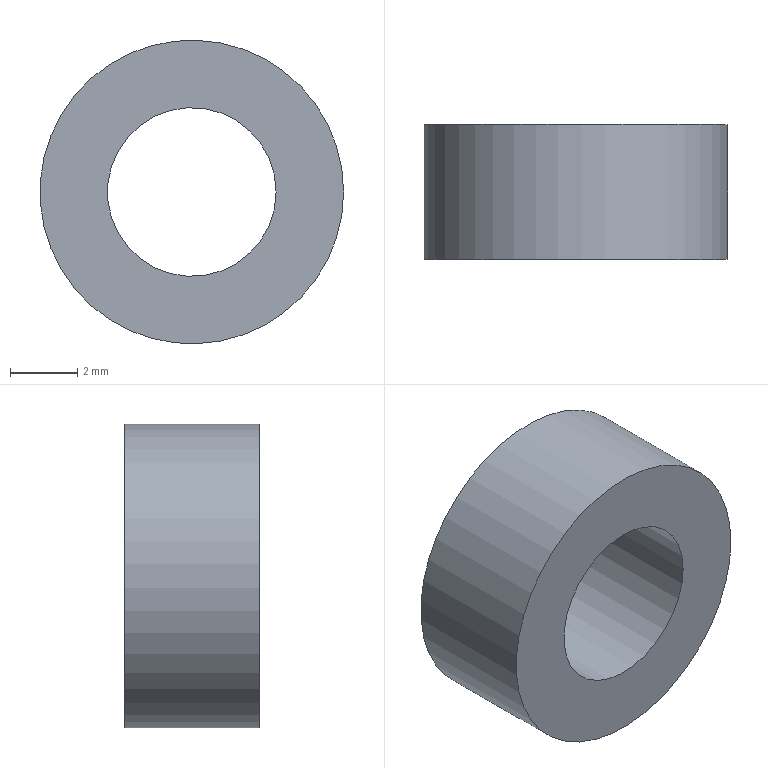Part | STEP file | 1-69.2 | 1 solid | 4 faces | box 9 x 4 x 9 mm | volume 175.929 mm3 | plane 2 | cylinder 2 | commonest cylinder face diameters 5 x1 9 x1
STEP:
#1=CARTESIAN_POINT('',(0.,0.,0.));
#2=DIRECTION('',(0.,0.,1.));
#3=DIRECTION('',(1.,0.,0.));
#4=AXIS2_PLACEMENT_3D('',#1,#2,#3);
#5=CARTESIAN_POINT('',(4.5,-2.,0.));
#6=VERTEX_POINT('',#5);
#7=CARTESIAN_POINT('',(0.,-2.,0.));
#8=DIRECTION('',(0.,-1.,0.));
#9=DIRECTION('',(1.,0.,0.));
#10=AXIS2_PLACEMENT_3D('',#7,#8,#9);
#11=CIRCLE('',#10,4.5);
#12=CARTESIAN_POINT('',(-1.206,-2.,0.));
#13=DIRECTION('',(0.,-1.,0.));
#14=DIRECTION('',(1.,0.,0.));
#15=AXIS2_PLACEMENT_3D('',#12,#13,#14);
#16=PLANE('',#15);
#17=CARTESIAN_POINT('',(1.206,0.));
#18=DIRECTION('',(1.,0.));
#19=AXIS2_PLACEMENT_2D('',#17,#18);
#20=CIRCLE('',#19,4.5);
#21=(GEOMETRIC_REPRESENTATION_CONTEXT(2)PARAMETRIC_REPRESENTATION_CONTEXT()REPRESENTATION_CONTEXT('',''));
#22=DEFINITIONAL_REPRESENTATION('',(#20),#21);
#23=PCURVE('',#16,#22);
#24=CARTESIAN_POINT('',(0.,-2.,0.));
#25=DIRECTION('',(0.,1.,0.));
#26=DIRECTION('',(1.,0.,0.));
#27=AXIS2_PLACEMENT_3D('',#24,#25,#26);
#28=CYLINDRICAL_SURFACE('',#27,4.5);
#29=CARTESIAN_POINT('',(6.283,0.));
#30=DIRECTION('',(-1.,0.));
#31=VECTOR('',#30,1.);
#32=LINE('',#29,#31);
#33=(GEOMETRIC_REPRESENTATION_CONTEXT(2)PARAMETRIC_REPRESENTATION_CONTEXT()REPRESENTATION_CONTEXT('',''));
#34=DEFINITIONAL_REPRESENTATION('',(#32),#33);
#35=PCURVE('',#28,#34);
#36=SURFACE_CURVE('',#11,(#23,#35),.PCURVE_S1.);
#37=EDGE_CURVE('',#6,#6,#36,.T.);
#38=ORIENTED_EDGE('',*,*,#37,.T.);
#39=EDGE_LOOP('',(#38));
#40=FACE_BOUND('',#39,.T.);
#41=CARTESIAN_POINT('',(2.5,-2.,0.));
#42=VERTEX_POINT('',#41);
#43=CARTESIAN_POINT('',(0.,-2.,0.));
#44=DIRECTION('',(0.,1.,0.));
#45=DIRECTION('',(1.,0.,0.));
#46=AXIS2_PLACEMENT_3D('',#43,#44,#45);
#47=CIRCLE('',#46,2.5);
#48=CARTESIAN_POINT('',(3.706,0.));
#49=CARTESIAN_POINT('',(3.706,-4.33));
#50=CARTESIAN_POINT('',(-0.04423,-2.165));
#51=CARTESIAN_POINT('',(-3.794,0.));
#52=CARTESIAN_POINT('',(-0.04423,2.165));
#53=CARTESIAN_POINT('',(3.706,4.33));
#54=CARTESIAN_POINT('',(3.706,0.));
#55=(BOUNDED_CURVE()B_SPLINE_CURVE(2,(#48,#49,#50,#51,#52,#53,#54),.UNSPECIFIED.,.T.,.F.)B_SPLINE_CURVE_WITH_KNOTS((1,2,2,2,2,1),(-2.094,0.,2.094,4.189,6.283,8.378),.UNSPECIFIED.)CURVE()GEOMETRIC_REPRESENTATION_ITEM()RATIONAL_B_SPLINE_CURVE((1.,0.5,1.,0.5,1.,0.5,1.))REPRESENTATION_ITEM(''));
#56=(GEOMETRIC_REPRESENTATION_CONTEXT(2)PARAMETRIC_REPRESENTATION_CONTEXT()REPRESENTATION_CONTEXT('',''));
#57=DEFINITIONAL_REPRESENTATION('',(#55),#56);
#58=PCURVE('',#16,#57);
#59=CARTESIAN_POINT('',(0.,-2.,0.));
#60=DIRECTION('',(0.,1.,0.));
#61=DIRECTION('',(1.,0.,0.));
#62=AXIS2_PLACEMENT_3D('',#59,#60,#61);
#63=CYLINDRICAL_SURFACE('',#62,2.5);
#64=CARTESIAN_POINT('',(0.,0.));
#65=DIRECTION('',(1.,0.));
#66=VECTOR('',#65,1.);
#67=LINE('',#64,#66);
#68=(GEOMETRIC_REPRESENTATION_CONTEXT(2)PARAMETRIC_REPRESENTATION_CONTEXT()REPRESENTATION_CONTEXT('',''));
#69=DEFINITIONAL_REPRESENTATION('',(#67),#68);
#70=PCURVE('',#63,#69);
#71=SURFACE_CURVE('',#47,(#58,#70),.PCURVE_S1.);
#72=EDGE_CURVE('',#42,#42,#71,.T.);
#73=ORIENTED_EDGE('',*,*,#72,.T.);
#74=EDGE_LOOP('',(#73));
#75=FACE_BOUND('',#74,.T.);
#76=ADVANCED_FACE('',(#40,#75),#16,.T.);
#77=CARTESIAN_POINT('',(4.5,2.,0.));
#78=VERTEX_POINT('',#77);
#79=CARTESIAN_POINT('',(0.,2.,0.));
#80=DIRECTION('',(0.,-1.,0.));
#81=DIRECTION('',(1.,0.,0.));
#82=AXIS2_PLACEMENT_3D('',#79,#80,#81);
#83=CIRCLE('',#82,4.5);
#84=CARTESIAN_POINT('',(-1.206,2.,0.));
#85=DIRECTION('',(0.,-1.,0.));
#86=DIRECTION('',(1.,0.,0.));
#87=AXIS2_PLACEMENT_3D('',#84,#85,#86);
#88=PLANE('',#87);
#89=CARTESIAN_POINT('',(1.206,0.));
#90=DIRECTION('',(1.,0.));
#91=AXIS2_PLACEMENT_2D('',#89,#90);
#92=CIRCLE('',#91,4.5);
#93=(GEOMETRIC_REPRESENTATION_CONTEXT(2)PARAMETRIC_REPRESENTATION_CONTEXT()REPRESENTATION_CONTEXT('',''));
#94=DEFINITIONAL_REPRESENTATION('',(#92),#93);
#95=PCURVE('',#88,#94);
#96=CARTESIAN_POINT('',(6.283,4.));
#97=DIRECTION('',(-1.,0.));
#98=VECTOR('',#97,1.);
#99=LINE('',#96,#98);
#100=(GEOMETRIC_REPRESENTATION_CONTEXT(2)PARAMETRIC_REPRESENTATION_CONTEXT()REPRESENTATION_CONTEXT('',''));
#101=DEFINITIONAL_REPRESENTATION('',(#99),#100);
#102=PCURVE('',#28,#101);
#103=SURFACE_CURVE('',#83,(#95,#102),.PCURVE_S1.);
#104=EDGE_CURVE('',#78,#78,#103,.T.);
#105=ORIENTED_EDGE('',*,*,#104,.T.);
#106=EDGE_LOOP('',(#105));
#107=FACE_BOUND('',#106,.F.);
#108=CARTESIAN_POINT('',(2.5,2.,0.));
#109=VERTEX_POINT('',#108);
#110=CARTESIAN_POINT('',(0.,2.,0.));
#111=DIRECTION('',(0.,1.,0.));
#112=DIRECTION('',(1.,0.,0.));
#113=AXIS2_PLACEMENT_3D('',#110,#111,#112);
#114=CIRCLE('',#113,2.5);
#115=CARTESIAN_POINT('',(3.706,0.));
#116=CARTESIAN_POINT('',(3.706,-4.33));
#117=CARTESIAN_POINT('',(-0.04423,-2.165));
#118=CARTESIAN_POINT('',(-3.794,0.));
#119=CARTESIAN_POINT('',(-0.04423,2.165));
#120=CARTESIAN_POINT('',(3.706,4.33));
#121=CARTESIAN_POINT('',(3.706,0.));
#122=(BOUNDED_CURVE()B_SPLINE_CURVE(2,(#115,#116,#117,#118,#119,#120,#121),.UNSPECIFIED.,.T.,.F.)B_SPLINE_CURVE_WITH_KNOTS((1,2,2,2,2,1),(-2.094,0.,2.094,4.189,6.283,8.378),.UNSPECIFIED.)CURVE()GEOMETRIC_REPRESENTATION_ITEM()RATIONAL_B_SPLINE_CURVE((1.,0.5,1.,0.5,1.,0.5,1.))REPRESENTATION_ITEM(''));
#123=(GEOMETRIC_REPRESENTATION_CONTEXT(2)PARAMETRIC_REPRESENTATION_CONTEXT()REPRESENTATION_CONTEXT('',''));
#124=DEFINITIONAL_REPRESENTATION('',(#122),#123);
#125=PCURVE('',#88,#124);
#126=CARTESIAN_POINT('',(0.,4.));
#127=DIRECTION('',(1.,0.));
#128=VECTOR('',#127,1.);
#129=LINE('',#126,#128);
#130=(GEOMETRIC_REPRESENTATION_CONTEXT(2)PARAMETRIC_REPRESENTATION_CONTEXT()REPRESENTATION_CONTEXT('',''));
#131=DEFINITIONAL_REPRESENTATION('',(#129),#130);
#132=PCURVE('',#63,#131);
#133=SURFACE_CURVE('',#114,(#125,#132),.PCURVE_S1.);
#134=EDGE_CURVE('',#109,#109,#133,.T.);
#135=ORIENTED_EDGE('',*,*,#134,.T.);
#136=EDGE_LOOP('',(#135));
#137=FACE_BOUND('',#136,.F.);
#138=ADVANCED_FACE('',(#107,#137),#88,.F.);
#139=CARTESIAN_POINT('',(4.5,-2.,0.));
#140=DIRECTION('',(0.,1.,0.));
#141=VECTOR('',#140,1.);
#142=LINE('',#139,#141);
#143=CARTESIAN_POINT('',(6.283,0.));
#144=DIRECTION('',(0.,1.));
#145=VECTOR('',#144,1.);
#146=LINE('',#143,#145);
#147=(GEOMETRIC_REPRESENTATION_CONTEXT(2)PARAMETRIC_REPRESENTATION_CONTEXT()REPRESENTATION_CONTEXT('',''));
#148=DEFINITIONAL_REPRESENTATION('',(#146),#147);
#149=PCURVE('',#28,#148);
#150=CARTESIAN_POINT('',(0.,0.));
#151=DIRECTION('',(0.,1.));
#152=VECTOR('',#151,1.);
#153=LINE('',#150,#152);
#154=(GEOMETRIC_REPRESENTATION_CONTEXT(2)PARAMETRIC_REPRESENTATION_CONTEXT()REPRESENTATION_CONTEXT('',''));
#155=DEFINITIONAL_REPRESENTATION('',(#153),#154);
#156=PCURVE('',#28,#155);
#157=SEAM_CURVE('',#142,(#149,#156),.PCURVE_S1.);
#158=EDGE_CURVE('',#6,#78,#157,.T.);
#159=ORIENTED_EDGE('',*,*,#158,.T.);
#160=ORIENTED_EDGE('',*,*,#104,.T.);
#161=ORIENTED_EDGE('',*,*,#158,.F.);
#162=ORIENTED_EDGE('',*,*,#37,.F.);
#163=EDGE_LOOP('',(#159,#160,#161,#162));
#164=FACE_BOUND('',#163,.T.);
#165=ADVANCED_FACE('',(#164),#28,.T.);
#166=ORIENTED_EDGE('',*,*,#72,.T.);
#167=CARTESIAN_POINT('',(2.5,-2.,0.));
#168=DIRECTION('',(0.,1.,0.));
#169=VECTOR('',#168,1.);
#170=LINE('',#167,#169);
#171=CARTESIAN_POINT('',(6.283,0.));
#172=DIRECTION('',(0.,1.));
#173=VECTOR('',#172,1.);
#174=LINE('',#171,#173);
#175=(GEOMETRIC_REPRESENTATION_CONTEXT(2)PARAMETRIC_REPRESENTATION_CONTEXT()REPRESENTATION_CONTEXT('',''));
#176=DEFINITIONAL_REPRESENTATION('',(#174),#175);
#177=PCURVE('',#63,#176);
#178=CARTESIAN_POINT('',(0.,0.));
#179=DIRECTION('',(0.,1.));
#180=VECTOR('',#179,1.);
#181=LINE('',#178,#180);
#182=(GEOMETRIC_REPRESENTATION_CONTEXT(2)PARAMETRIC_REPRESENTATION_CONTEXT()REPRESENTATION_CONTEXT('',''));
#183=DEFINITIONAL_REPRESENTATION('',(#181),#182);
#184=PCURVE('',#63,#183);
#185=SEAM_CURVE('',#170,(#177,#184),.PCURVE_S1.);
#186=EDGE_CURVE('',#42,#109,#185,.T.);
#187=ORIENTED_EDGE('',*,*,#186,.T.);
#188=ORIENTED_EDGE('',*,*,#134,.F.);
#189=ORIENTED_EDGE('',*,*,#186,.F.);
#190=EDGE_LOOP('',(#166,#187,#188,#189));
#191=FACE_BOUND('',#190,.F.);
#192=ADVANCED_FACE('',(#191),#63,.F.);
#193=CLOSED_SHELL('',(#76,#138,#165,#192));
#194=MANIFOLD_SOLID_BREP('',#193);
#195=(LENGTH_UNIT()NAMED_UNIT(*)SI_UNIT(.MILLI.,.METRE.));
#196=UNCERTAINTY_MEASURE_WITH_UNIT(LENGTH_MEASURE(0.0000001),#195,'','');
#197=(NAMED_UNIT(*)PLANE_ANGLE_UNIT()SI_UNIT($,.RADIAN.));
#198=(NAMED_UNIT(*)SI_UNIT($,.STERADIAN.)SOLID_ANGLE_UNIT());
#199=(GEOMETRIC_REPRESENTATION_CONTEXT(3)GLOBAL_UNCERTAINTY_ASSIGNED_CONTEXT((#196))GLOBAL_UNIT_ASSIGNED_CONTEXT((#195,#197,#198))REPRESENTATION_CONTEXT('',''));
#200=ADVANCED_BREP_SHAPE_REPRESENTATION('',(#4,#194),#199);